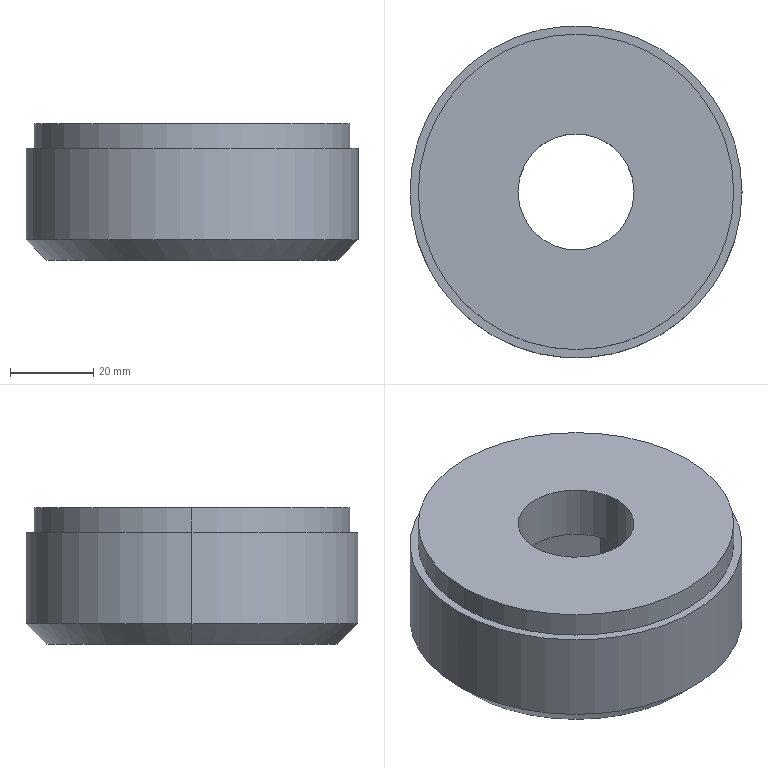Part | SolidWorks | features ICE 3, Chamfer 1, Extrusion 1 | 1 solid | 18 faces | box 80 x 80 x 33 mm | volume 125576 mm3 | plane 10 | cylinder 6 | cone 2 | commonest cylinder face diameters 28 x2 76 x2 80 x2
STEP:
#1=CARTESIAN_POINT('',(-14.,0.,20.));
#2=VERTEX_POINT('',#1);
#3=CARTESIAN_POINT('',(14.,0.,20.));
#4=VERTEX_POINT('',#3);
#5=CARTESIAN_POINT('',(0.,0.,20.));
#6=DIRECTION('',(0.,0.,1.));
#7=DIRECTION('',(-1.,0.,0.));
#8=AXIS2_PLACEMENT_3D('',#5,#6,#7);
#9=CIRCLE('',#8,14.);
#10=EDGE_CURVE('',#2,#4,#9,.T.);
#11=ORIENTED_EDGE('',*,*,#10,.F.);
#12=CARTESIAN_POINT('',(-14.,0.,33.));
#13=VERTEX_POINT('',#12);
#14=CARTESIAN_POINT('',(-14.,0.,20.));
#15=DIRECTION('',(0.,0.,1.));
#16=VECTOR('',#15,1000.);
#17=LINE('',#14,#16);
#18=EDGE_CURVE('',#2,#13,#17,.T.);
#19=ORIENTED_EDGE('',*,*,#18,.T.);
#20=CARTESIAN_POINT('',(14.,0.,33.));
#21=VERTEX_POINT('',#20);
#22=CARTESIAN_POINT('',(0.,0.,33.));
#23=DIRECTION('',(0.,0.,1.));
#24=DIRECTION('',(1.,0.,0.));
#25=AXIS2_PLACEMENT_3D('',#22,#23,#24);
#26=CIRCLE('',#25,14.);
#27=EDGE_CURVE('',#13,#21,#26,.T.);
#28=ORIENTED_EDGE('',*,*,#27,.T.);
#29=CARTESIAN_POINT('',(14.,0.,20.));
#30=DIRECTION('',(0.,0.,1.));
#31=VECTOR('',#30,1000.);
#32=LINE('',#29,#31);
#33=EDGE_CURVE('',#4,#21,#32,.T.);
#34=ORIENTED_EDGE('',*,*,#33,.F.);
#35=EDGE_LOOP('',(#11,#19,#28,#34));
#36=FACE_OUTER_BOUND('',#35,.T.);
#37=CARTESIAN_POINT('',(0.,0.,20.));
#38=DIRECTION('',(0.,0.,1.));
#39=DIRECTION('',(1.,0.,0.));
#40=AXIS2_PLACEMENT_3D('',#37,#38,#39);
#41=CYLINDRICAL_SURFACE('',#40,14.);
#42=ADVANCED_FACE('',(#36),#41,.F.);
#43=CARTESIAN_POINT('',(-35.,0.,0.));
#44=VERTEX_POINT('',#43);
#45=CARTESIAN_POINT('',(35.,0.,0.));
#46=VERTEX_POINT('',#45);
#47=CARTESIAN_POINT('',(0.,0.,0.));
#48=DIRECTION('',(0.,0.,-1.));
#49=DIRECTION('',(1.,0.,0.));
#50=AXIS2_PLACEMENT_3D('',#47,#48,#49);
#51=CIRCLE('',#50,35.);
#52=EDGE_CURVE('',#44,#46,#51,.T.);
#53=ORIENTED_EDGE('',*,*,#52,.F.);
#54=CARTESIAN_POINT('',(-40.,0.,5.));
#55=VERTEX_POINT('',#54);
#56=CARTESIAN_POINT('',(-40.,0.,5.));
#57=DIRECTION('',(-0.7071,0.,0.7071));
#58=VECTOR('',#57,1000.);
#59=LINE('',#56,#58);
#60=EDGE_CURVE('',#44,#55,#59,.T.);
#61=ORIENTED_EDGE('',*,*,#60,.T.);
#62=CARTESIAN_POINT('',(40.,0.,5.));
#63=VERTEX_POINT('',#62);
#64=CARTESIAN_POINT('',(0.,0.,5.));
#65=DIRECTION('',(0.,0.,1.));
#66=DIRECTION('',(1.,0.,0.));
#67=AXIS2_PLACEMENT_3D('',#64,#65,#66);
#68=CIRCLE('',#67,40.);
#69=EDGE_CURVE('',#63,#55,#68,.T.);
#70=ORIENTED_EDGE('',*,*,#69,.F.);
#71=CARTESIAN_POINT('',(40.,0.,5.));
#72=DIRECTION('',(0.7071,0.,0.7071));
#73=VECTOR('',#72,1000.);
#74=LINE('',#71,#73);
#75=EDGE_CURVE('',#46,#63,#74,.T.);
#76=ORIENTED_EDGE('',*,*,#75,.F.);
#77=EDGE_LOOP('',(#53,#61,#70,#76));
#78=FACE_OUTER_BOUND('',#77,.T.);
#79=CARTESIAN_POINT('',(0.,0.,5.));
#80=DIRECTION('',(0.,0.,1.));
#81=DIRECTION('',(1.,0.,0.));
#82=AXIS2_PLACEMENT_3D('',#79,#80,#81);
#83=CONICAL_SURFACE('',#82,40.,0.7854);
#84=ADVANCED_FACE('',(#78),#83,.T.);
#85=CARTESIAN_POINT('',(38.,0.,27.));
#86=VERTEX_POINT('',#85);
#87=CARTESIAN_POINT('',(-38.,0.,27.));
#88=VERTEX_POINT('',#87);
#89=CARTESIAN_POINT('',(0.,0.,27.));
#90=DIRECTION('',(0.,0.,1.));
#91=DIRECTION('',(1.,0.,0.));
#92=AXIS2_PLACEMENT_3D('',#89,#90,#91);
#93=CIRCLE('',#92,38.);
#94=EDGE_CURVE('',#86,#88,#93,.T.);
#95=ORIENTED_EDGE('',*,*,#94,.T.);
#96=CARTESIAN_POINT('',(-38.,0.,33.));
#97=VERTEX_POINT('',#96);
#98=CARTESIAN_POINT('',(-38.,0.,27.));
#99=DIRECTION('',(0.,0.,1.));
#100=VECTOR('',#99,1000.);
#101=LINE('',#98,#100);
#102=EDGE_CURVE('',#88,#97,#101,.T.);
#103=ORIENTED_EDGE('',*,*,#102,.T.);
#104=CARTESIAN_POINT('',(38.,0.,33.));
#105=VERTEX_POINT('',#104);
#106=CARTESIAN_POINT('',(0.,0.,33.));
#107=DIRECTION('',(0.,0.,1.));
#108=DIRECTION('',(1.,0.,0.));
#109=AXIS2_PLACEMENT_3D('',#106,#107,#108);
#110=CIRCLE('',#109,38.);
#111=EDGE_CURVE('',#105,#97,#110,.T.);
#112=ORIENTED_EDGE('',*,*,#111,.F.);
#113=CARTESIAN_POINT('',(38.,0.,27.));
#114=DIRECTION('',(0.,0.,1.));
#115=VECTOR('',#114,1000.);
#116=LINE('',#113,#115);
#117=EDGE_CURVE('',#86,#105,#116,.T.);
#118=ORIENTED_EDGE('',*,*,#117,.F.);
#119=EDGE_LOOP('',(#95,#103,#112,#118));
#120=FACE_OUTER_BOUND('',#119,.T.);
#121=CARTESIAN_POINT('',(0.,0.,27.));
#122=DIRECTION('',(0.,0.,1.));
#123=DIRECTION('',(1.,0.,0.));
#124=AXIS2_PLACEMENT_3D('',#121,#122,#123);
#125=CYLINDRICAL_SURFACE('',#124,38.);
#126=ADVANCED_FACE('',(#120),#125,.T.);
#127=CARTESIAN_POINT('',(40.,0.,27.));
#128=VERTEX_POINT('',#127);
#129=CARTESIAN_POINT('',(-40.,0.,27.));
#130=VERTEX_POINT('',#129);
#131=CARTESIAN_POINT('',(0.,0.,27.));
#132=DIRECTION('',(0.,0.,1.));
#133=DIRECTION('',(1.,0.,0.));
#134=AXIS2_PLACEMENT_3D('',#131,#132,#133);
#135=CIRCLE('',#134,40.);
#136=EDGE_CURVE('',#128,#130,#135,.T.);
#137=ORIENTED_EDGE('',*,*,#136,.F.);
#138=CARTESIAN_POINT('',(40.,0.,33.));
#139=DIRECTION('',(0.,0.,-1.));
#140=VECTOR('',#139,1000.);
#141=LINE('',#138,#140);
#142=EDGE_CURVE('',#128,#63,#141,.T.);
#143=ORIENTED_EDGE('',*,*,#142,.T.);
#144=ORIENTED_EDGE('',*,*,#69,.T.);
#145=CARTESIAN_POINT('',(-40.,0.,33.));
#146=DIRECTION('',(0.,0.,-1.));
#147=VECTOR('',#146,1000.);
#148=LINE('',#145,#147);
#149=EDGE_CURVE('',#130,#55,#148,.T.);
#150=ORIENTED_EDGE('',*,*,#149,.F.);
#151=EDGE_LOOP('',(#137,#143,#144,#150));
#152=FACE_OUTER_BOUND('',#151,.T.);
#153=CARTESIAN_POINT('',(0.,0.,33.));
#154=DIRECTION('',(0.,0.,-1.));
#155=DIRECTION('',(-1.,0.,0.));
#156=AXIS2_PLACEMENT_3D('',#153,#154,#155);
#157=CYLINDRICAL_SURFACE('',#156,40.);
#158=ADVANCED_FACE('',(#152),#157,.T.);
#159=ORIENTED_EDGE('',*,*,#142,.F.);
#160=CARTESIAN_POINT('',(0.,0.,27.));
#161=DIRECTION('',(0.,0.,1.));
#162=DIRECTION('',(1.,0.,0.));
#163=AXIS2_PLACEMENT_3D('',#160,#161,#162);
#164=CIRCLE('',#163,40.);
#165=EDGE_CURVE('',#130,#128,#164,.T.);
#166=ORIENTED_EDGE('',*,*,#165,.F.);
#167=ORIENTED_EDGE('',*,*,#149,.T.);
#168=CARTESIAN_POINT('',(0.,0.,5.));
#169=DIRECTION('',(0.,0.,1.));
#170=DIRECTION('',(1.,0.,0.));
#171=AXIS2_PLACEMENT_3D('',#168,#169,#170);
#172=CIRCLE('',#171,40.);
#173=EDGE_CURVE('',#55,#63,#172,.T.);
#174=ORIENTED_EDGE('',*,*,#173,.T.);
#175=EDGE_LOOP('',(#159,#166,#167,#174));
#176=FACE_OUTER_BOUND('',#175,.T.);
#177=CARTESIAN_POINT('',(0.,0.,33.));
#178=DIRECTION('',(0.,0.,-1.));
#179=DIRECTION('',(-1.,0.,0.));
#180=AXIS2_PLACEMENT_3D('',#177,#178,#179);
#181=CYLINDRICAL_SURFACE('',#180,40.);
#182=ADVANCED_FACE('',(#176),#181,.T.);
#183=CARTESIAN_POINT('',(19.5,-11.258,0.));
#184=VERTEX_POINT('',#183);
#185=CARTESIAN_POINT('',(0.,-22.517,0.));
#186=VERTEX_POINT('',#185);
#187=CARTESIAN_POINT('',(19.5,-11.258,0.));
#188=DIRECTION('',(-0.866,-0.5,0.));
#189=VECTOR('',#188,1000.);
#190=LINE('',#187,#189);
#191=EDGE_CURVE('',#184,#186,#190,.T.);
#192=ORIENTED_EDGE('',*,*,#191,.F.);
#193=CARTESIAN_POINT('',(19.5,11.258,0.));
#194=VERTEX_POINT('',#193);
#195=CARTESIAN_POINT('',(19.5,11.258,0.));
#196=DIRECTION('',(0.,-1.,0.));
#197=VECTOR('',#196,1000.);
#198=LINE('',#195,#197);
#199=EDGE_CURVE('',#194,#184,#198,.T.);
#200=ORIENTED_EDGE('',*,*,#199,.F.);
#201=CARTESIAN_POINT('',(0.,22.517,0.));
#202=VERTEX_POINT('',#201);
#203=CARTESIAN_POINT('',(0.,22.517,0.));
#204=DIRECTION('',(0.866,-0.5,0.));
#205=VECTOR('',#204,1000.);
#206=LINE('',#203,#205);
#207=EDGE_CURVE('',#202,#194,#206,.T.);
#208=ORIENTED_EDGE('',*,*,#207,.F.);
#209=CARTESIAN_POINT('',(-19.5,11.258,0.));
#210=VERTEX_POINT('',#209);
#211=CARTESIAN_POINT('',(-19.5,11.258,0.));
#212=DIRECTION('',(0.866,0.5,0.));
#213=VECTOR('',#212,1000.);
#214=LINE('',#211,#213);
#215=EDGE_CURVE('',#210,#202,#214,.T.);
#216=ORIENTED_EDGE('',*,*,#215,.F.);
#217=CARTESIAN_POINT('',(-19.5,-11.258,0.));
#218=VERTEX_POINT('',#217);
#219=CARTESIAN_POINT('',(-19.5,-11.258,0.));
#220=DIRECTION('',(0.,1.,0.));
#221=VECTOR('',#220,1000.);
#222=LINE('',#219,#221);
#223=EDGE_CURVE('',#218,#210,#222,.T.);
#224=ORIENTED_EDGE('',*,*,#223,.F.);
#225=CARTESIAN_POINT('',(0.,-22.517,0.));
#226=DIRECTION('',(-0.866,0.5,0.));
#227=VECTOR('',#226,1000.);
#228=LINE('',#225,#227);
#229=EDGE_CURVE('',#186,#218,#228,.T.);
#230=ORIENTED_EDGE('',*,*,#229,.F.);
#231=EDGE_LOOP('',(#192,#200,#208,#216,#224,#230));
#232=FACE_BOUND('',#231,.T.);
#233=CARTESIAN_POINT('',(0.,0.,0.));
#234=DIRECTION('',(0.,0.,-1.));
#235=DIRECTION('',(1.,0.,0.));
#236=AXIS2_PLACEMENT_3D('',#233,#234,#235);
#237=CIRCLE('',#236,35.);
#238=EDGE_CURVE('',#46,#44,#237,.T.);
#239=ORIENTED_EDGE('',*,*,#238,.T.);
#240=ORIENTED_EDGE('',*,*,#52,.T.);
#241=EDGE_LOOP('',(#239,#240));
#242=FACE_OUTER_BOUND('',#241,.T.);
#243=CARTESIAN_POINT('',(0.,0.,0.));
#244=DIRECTION('',(0.,0.,1.));
#245=DIRECTION('',(1.,0.,0.));
#246=AXIS2_PLACEMENT_3D('',#243,#244,#245);
#247=PLANE('',#246);
#248=ADVANCED_FACE('',(#232,#242),#247,.F.);
#249=ORIENTED_EDGE('',*,*,#94,.F.);
#250=CARTESIAN_POINT('',(0.,0.,27.));
#251=DIRECTION('',(0.,0.,1.));
#252=DIRECTION('',(1.,0.,0.));
#253=AXIS2_PLACEMENT_3D('',#250,#251,#252);
#254=CIRCLE('',#253,38.);
#255=EDGE_CURVE('',#88,#86,#254,.T.);
#256=ORIENTED_EDGE('',*,*,#255,.F.);
#257=EDGE_LOOP('',(#249,#256));
#258=FACE_BOUND('',#257,.T.);
#259=ORIENTED_EDGE('',*,*,#165,.T.);
#260=ORIENTED_EDGE('',*,*,#136,.T.);
#261=EDGE_LOOP('',(#259,#260));
#262=FACE_OUTER_BOUND('',#261,.T.);
#263=CARTESIAN_POINT('',(0.,0.,27.));
#264=DIRECTION('',(0.,0.,1.));
#265=DIRECTION('',(1.,0.,0.));
#266=AXIS2_PLACEMENT_3D('',#263,#264,#265);
#267=PLANE('',#266);
#268=ADVANCED_FACE('',(#258,#262),#267,.T.);
#269=ORIENTED_EDGE('',*,*,#102,.F.);
#270=ORIENTED_EDGE('',*,*,#255,.T.);
#271=ORIENTED_EDGE('',*,*,#117,.T.);
#272=CARTESIAN_POINT('',(0.,0.,33.));
#273=DIRECTION('',(0.,0.,1.));
#274=DIRECTION('',(1.,0.,0.));
#275=AXIS2_PLACEMENT_3D('',#272,#273,#274);
#276=CIRCLE('',#275,38.);
#277=EDGE_CURVE('',#97,#105,#276,.T.);
#278=ORIENTED_EDGE('',*,*,#277,.F.);
#279=EDGE_LOOP('',(#269,#270,#271,#278));
#280=FACE_OUTER_BOUND('',#279,.T.);
#281=CARTESIAN_POINT('',(0.,0.,27.));
#282=DIRECTION('',(0.,0.,1.));
#283=DIRECTION('',(1.,0.,0.));
#284=AXIS2_PLACEMENT_3D('',#281,#282,#283);
#285=CYLINDRICAL_SURFACE('',#284,38.);
#286=ADVANCED_FACE('',(#280),#285,.T.);
#287=CARTESIAN_POINT('',(0.,0.,33.));
#288=DIRECTION('',(0.,0.,1.));
#289=DIRECTION('',(1.,0.,0.));
#290=AXIS2_PLACEMENT_3D('',#287,#288,#289);
#291=CIRCLE('',#290,14.);
#292=EDGE_CURVE('',#21,#13,#291,.T.);
#293=ORIENTED_EDGE('',*,*,#292,.F.);
#294=ORIENTED_EDGE('',*,*,#27,.F.);
#295=EDGE_LOOP('',(#293,#294));
#296=FACE_BOUND('',#295,.T.);
#297=ORIENTED_EDGE('',*,*,#111,.T.);
#298=ORIENTED_EDGE('',*,*,#277,.T.);
#299=EDGE_LOOP('',(#297,#298));
#300=FACE_OUTER_BOUND('',#299,.T.);
#301=CARTESIAN_POINT('',(0.,0.,33.));
#302=DIRECTION('',(0.,0.,1.));
#303=DIRECTION('',(1.,0.,0.));
#304=AXIS2_PLACEMENT_3D('',#301,#302,#303);
#305=PLANE('',#304);
#306=ADVANCED_FACE('',(#296,#300),#305,.T.);
#307=ORIENTED_EDGE('',*,*,#60,.F.);
#308=ORIENTED_EDGE('',*,*,#238,.F.);
#309=ORIENTED_EDGE('',*,*,#75,.T.);
#310=ORIENTED_EDGE('',*,*,#173,.F.);
#311=EDGE_LOOP('',(#307,#308,#309,#310));
#312=FACE_OUTER_BOUND('',#311,.T.);
#313=CARTESIAN_POINT('',(0.,0.,5.));
#314=DIRECTION('',(0.,0.,1.));
#315=DIRECTION('',(1.,0.,0.));
#316=AXIS2_PLACEMENT_3D('',#313,#314,#315);
#317=CONICAL_SURFACE('',#316,40.,0.7854);
#318=ADVANCED_FACE('',(#312),#317,.T.);
#319=ORIENTED_EDGE('',*,*,#18,.F.);
#320=CARTESIAN_POINT('',(0.,0.,20.));
#321=DIRECTION('',(0.,0.,1.));
#322=DIRECTION('',(-1.,0.,0.));
#323=AXIS2_PLACEMENT_3D('',#320,#321,#322);
#324=CIRCLE('',#323,14.);
#325=EDGE_CURVE('',#4,#2,#324,.T.);
#326=ORIENTED_EDGE('',*,*,#325,.F.);
#327=ORIENTED_EDGE('',*,*,#33,.T.);
#328=ORIENTED_EDGE('',*,*,#292,.T.);
#329=EDGE_LOOP('',(#319,#326,#327,#328));
#330=FACE_OUTER_BOUND('',#329,.T.);
#331=CARTESIAN_POINT('',(0.,0.,20.));
#332=DIRECTION('',(0.,0.,1.));
#333=DIRECTION('',(1.,0.,0.));
#334=AXIS2_PLACEMENT_3D('',#331,#332,#333);
#335=CYLINDRICAL_SURFACE('',#334,14.);
#336=ADVANCED_FACE('',(#330),#335,.F.);
#337=CARTESIAN_POINT('',(19.5,11.258,20.));
#338=VERTEX_POINT('',#337);
#339=CARTESIAN_POINT('',(19.5,-11.258,20.));
#340=VERTEX_POINT('',#339);
#341=CARTESIAN_POINT('',(19.5,11.258,20.));
#342=DIRECTION('',(0.,-1.,0.));
#343=VECTOR('',#342,1000.);
#344=LINE('',#341,#343);
#345=EDGE_CURVE('',#338,#340,#344,.T.);
#346=ORIENTED_EDGE('',*,*,#345,.T.);
#347=CARTESIAN_POINT('',(0.,-22.517,20.));
#348=VERTEX_POINT('',#347);
#349=CARTESIAN_POINT('',(19.5,-11.258,20.));
#350=DIRECTION('',(-0.866,-0.5,0.));
#351=VECTOR('',#350,1000.);
#352=LINE('',#349,#351);
#353=EDGE_CURVE('',#340,#348,#352,.T.);
#354=ORIENTED_EDGE('',*,*,#353,.T.);
#355=CARTESIAN_POINT('',(-19.5,-11.258,20.));
#356=VERTEX_POINT('',#355);
#357=CARTESIAN_POINT('',(0.,-22.517,20.));
#358=DIRECTION('',(-0.866,0.5,0.));
#359=VECTOR('',#358,1000.);
#360=LINE('',#357,#359);
#361=EDGE_CURVE('',#348,#356,#360,.T.);
#362=ORIENTED_EDGE('',*,*,#361,.T.);
#363=CARTESIAN_POINT('',(-19.5,11.258,20.));
#364=VERTEX_POINT('',#363);
#365=CARTESIAN_POINT('',(-19.5,-11.258,20.));
#366=DIRECTION('',(0.,1.,0.));
#367=VECTOR('',#366,1000.);
#368=LINE('',#365,#367);
#369=EDGE_CURVE('',#356,#364,#368,.T.);
#370=ORIENTED_EDGE('',*,*,#369,.T.);
#371=CARTESIAN_POINT('',(0.,22.517,20.));
#372=VERTEX_POINT('',#371);
#373=CARTESIAN_POINT('',(-19.5,11.258,20.));
#374=DIRECTION('',(0.866,0.5,0.));
#375=VECTOR('',#374,1000.);
#376=LINE('',#373,#375);
#377=EDGE_CURVE('',#364,#372,#376,.T.);
#378=ORIENTED_EDGE('',*,*,#377,.T.);
#379=CARTESIAN_POINT('',(0.,22.517,20.));
#380=DIRECTION('',(0.866,-0.5,0.));
#381=VECTOR('',#380,1000.);
#382=LINE('',#379,#381);
#383=EDGE_CURVE('',#372,#338,#382,.T.);
#384=ORIENTED_EDGE('',*,*,#383,.T.);
#385=EDGE_LOOP('',(#346,#354,#362,#370,#378,#384));
#386=FACE_OUTER_BOUND('',#385,.T.);
#387=ORIENTED_EDGE('',*,*,#325,.T.);
#388=ORIENTED_EDGE('',*,*,#10,.T.);
#389=EDGE_LOOP('',(#387,#388));
#390=FACE_BOUND('',#389,.T.);
#391=CARTESIAN_POINT('',(19.5,-11.258,20.));
#392=DIRECTION('',(0.,0.,-1.));
#393=DIRECTION('',(-1.,0.,0.));
#394=AXIS2_PLACEMENT_3D('',#391,#392,#393);
#395=PLANE('',#394);
#396=ADVANCED_FACE('',(#386,#390),#395,.T.);
#397=ORIENTED_EDGE('',*,*,#199,.T.);
#398=CARTESIAN_POINT('',(19.5,-11.258,20.));
#399=DIRECTION('',(0.,0.,-1.));
#400=VECTOR('',#399,1000.);
#401=LINE('',#398,#400);
#402=EDGE_CURVE('',#340,#184,#401,.T.);
#403=ORIENTED_EDGE('',*,*,#402,.F.);
#404=ORIENTED_EDGE('',*,*,#345,.F.);
#405=CARTESIAN_POINT('',(19.5,11.258,20.));
#406=DIRECTION('',(0.,0.,-1.));
#407=VECTOR('',#406,1000.);
#408=LINE('',#405,#407);
#409=EDGE_CURVE('',#338,#194,#408,.T.);
#410=ORIENTED_EDGE('',*,*,#409,.T.);
#411=EDGE_LOOP('',(#397,#403,#404,#410));
#412=FACE_OUTER_BOUND('',#411,.T.);
#413=CARTESIAN_POINT('',(19.5,11.258,20.));
#414=DIRECTION('',(1.,0.,0.));
#415=DIRECTION('',(0.,1.,0.));
#416=AXIS2_PLACEMENT_3D('',#413,#414,#415);
#417=PLANE('',#416);
#418=ADVANCED_FACE('',(#412),#417,.F.);
#419=ORIENTED_EDGE('',*,*,#207,.T.);
#420=ORIENTED_EDGE('',*,*,#409,.F.);
#421=ORIENTED_EDGE('',*,*,#383,.F.);
#422=CARTESIAN_POINT('',(0.,22.517,20.));
#423=DIRECTION('',(0.,0.,-1.));
#424=VECTOR('',#423,1000.);
#425=LINE('',#422,#424);
#426=EDGE_CURVE('',#372,#202,#425,.T.);
#427=ORIENTED_EDGE('',*,*,#426,.T.);
#428=EDGE_LOOP('',(#419,#420,#421,#427));
#429=FACE_OUTER_BOUND('',#428,.T.);
#430=CARTESIAN_POINT('',(0.,22.517,20.));
#431=DIRECTION('',(0.5,0.866,0.));
#432=DIRECTION('',(-0.866,0.5,0.));
#433=AXIS2_PLACEMENT_3D('',#430,#431,#432);
#434=PLANE('',#433);
#435=ADVANCED_FACE('',(#429),#434,.F.);
#436=ORIENTED_EDGE('',*,*,#215,.T.);
#437=ORIENTED_EDGE('',*,*,#426,.F.);
#438=ORIENTED_EDGE('',*,*,#377,.F.);
#439=CARTESIAN_POINT('',(-19.5,11.258,20.));
#440=DIRECTION('',(0.,0.,-1.));
#441=VECTOR('',#440,1000.);
#442=LINE('',#439,#441);
#443=EDGE_CURVE('',#364,#210,#442,.T.);
#444=ORIENTED_EDGE('',*,*,#443,.T.);
#445=EDGE_LOOP('',(#436,#437,#438,#444));
#446=FACE_OUTER_BOUND('',#445,.T.);
#447=CARTESIAN_POINT('',(-19.5,11.258,20.));
#448=DIRECTION('',(-0.5,0.866,0.));
#449=DIRECTION('',(-0.866,-0.5,0.));
#450=AXIS2_PLACEMENT_3D('',#447,#448,#449);
#451=PLANE('',#450);
#452=ADVANCED_FACE('',(#446),#451,.F.);
#453=ORIENTED_EDGE('',*,*,#223,.T.);
#454=ORIENTED_EDGE('',*,*,#443,.F.);
#455=ORIENTED_EDGE('',*,*,#369,.F.);
#456=CARTESIAN_POINT('',(-19.5,-11.258,20.));
#457=DIRECTION('',(0.,0.,-1.));
#458=VECTOR('',#457,1000.);
#459=LINE('',#456,#458);
#460=EDGE_CURVE('',#356,#218,#459,.T.);
#461=ORIENTED_EDGE('',*,*,#460,.T.);
#462=EDGE_LOOP('',(#453,#454,#455,#461));
#463=FACE_OUTER_BOUND('',#462,.T.);
#464=CARTESIAN_POINT('',(-19.5,-11.258,20.));
#465=DIRECTION('',(-1.,0.,0.));
#466=DIRECTION('',(0.,-1.,0.));
#467=AXIS2_PLACEMENT_3D('',#464,#465,#466);
#468=PLANE('',#467);
#469=ADVANCED_FACE('',(#463),#468,.F.);
#470=ORIENTED_EDGE('',*,*,#229,.T.);
#471=ORIENTED_EDGE('',*,*,#460,.F.);
#472=ORIENTED_EDGE('',*,*,#361,.F.);
#473=CARTESIAN_POINT('',(0.,-22.517,20.));
#474=DIRECTION('',(0.,0.,-1.));
#475=VECTOR('',#474,1000.);
#476=LINE('',#473,#475);
#477=EDGE_CURVE('',#348,#186,#476,.T.);
#478=ORIENTED_EDGE('',*,*,#477,.T.);
#479=EDGE_LOOP('',(#470,#471,#472,#478));
#480=FACE_OUTER_BOUND('',#479,.T.);
#481=CARTESIAN_POINT('',(0.,-22.517,20.));
#482=DIRECTION('',(-0.5,-0.866,0.));
#483=DIRECTION('',(0.866,-0.5,0.));
#484=AXIS2_PLACEMENT_3D('',#481,#482,#483);
#485=PLANE('',#484);
#486=ADVANCED_FACE('',(#480),#485,.F.);
#487=ORIENTED_EDGE('',*,*,#191,.T.);
#488=ORIENTED_EDGE('',*,*,#477,.F.);
#489=ORIENTED_EDGE('',*,*,#353,.F.);
#490=ORIENTED_EDGE('',*,*,#402,.T.);
#491=EDGE_LOOP('',(#487,#488,#489,#490));
#492=FACE_OUTER_BOUND('',#491,.T.);
#493=CARTESIAN_POINT('',(19.5,-11.258,20.));
#494=DIRECTION('',(0.5,-0.866,0.));
#495=DIRECTION('',(0.866,0.5,0.));
#496=AXIS2_PLACEMENT_3D('',#493,#494,#495);
#497=PLANE('',#496);
#498=ADVANCED_FACE('',(#492),#497,.F.);
#499=CLOSED_SHELL('',(#42,#84,#126,#158,#182,#248,#268,#286,#306,#318,#336,#396,#418,#435,#452,#469,#486,#498));
#500=MANIFOLD_SOLID_BREP('',#499);
#501=CARTESIAN_POINT('',(0.,0.,0.));
#502=DIRECTION('',(0.,0.,1.));
#503=DIRECTION('',(1.,0.,0.));
#504=AXIS2_PLACEMENT_3D('',#501,#502,#503);
#505=(LENGTH_UNIT()NAMED_UNIT(*)SI_UNIT(.MILLI.,.METRE.));
#506=UNCERTAINTY_MEASURE_WITH_UNIT(LENGTH_MEASURE(0.00001),#505,'','');
#507=(NAMED_UNIT(*)PLANE_ANGLE_UNIT()SI_UNIT($,.RADIAN.));
#508=(NAMED_UNIT(*)SI_UNIT($,.STERADIAN.)SOLID_ANGLE_UNIT());
#509=(GEOMETRIC_REPRESENTATION_CONTEXT(3)GLOBAL_UNCERTAINTY_ASSIGNED_CONTEXT((#506))GLOBAL_UNIT_ASSIGNED_CONTEXT((#505,#507,#508))REPRESENTATION_CONTEXT('',''));
#510=ADVANCED_BREP_SHAPE_REPRESENTATION('',(#500,#504),#509);